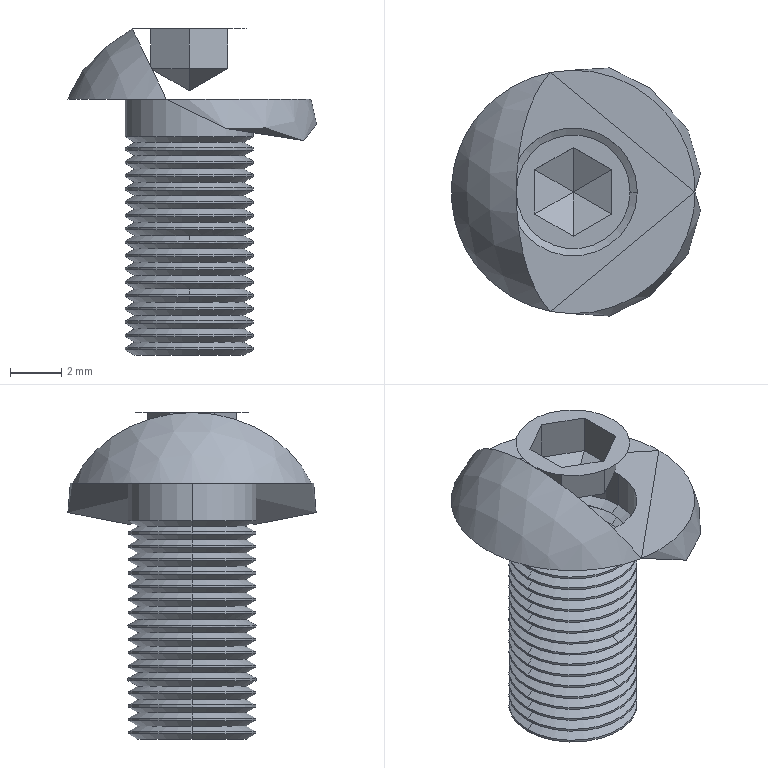Part | SolidWorks | features BaseBody 1 | 1 solid | 117 faces | volume 328.453 mm3 | cone 66 | cylinder 34 | plane 15 | sphere 2 | commonest cylinder face diameters 5 x34